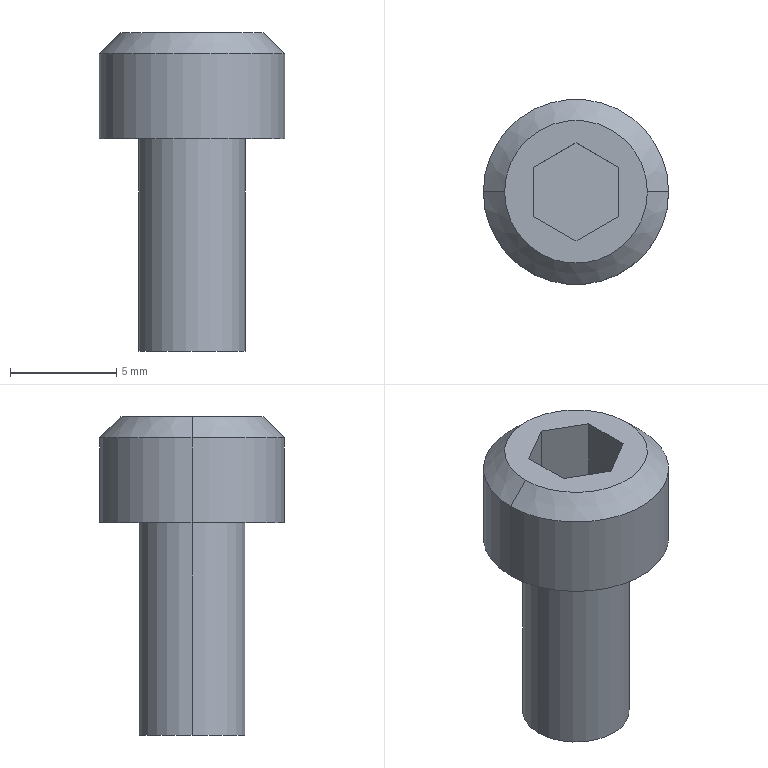Part | SolidWorks | features ICE 2, Chamfer 1, Extrusion 1 | 1 solid | 16 faces | box 8.72 x 8.72 x 15 mm | volume 426.876 mm3 | plane 10 | cylinder 4 | cone 2 | commonest cylinder face diameters 5 x2 8.72 x2
STEP:
#1=CARTESIAN_POINT('',(-2.5,0.,-10.));
#2=VERTEX_POINT('',#1);
#3=CARTESIAN_POINT('',(2.5,0.,-10.));
#4=VERTEX_POINT('',#3);
#5=CARTESIAN_POINT('',(0.,0.,-10.));
#6=DIRECTION('',(0.,0.,-1.));
#7=DIRECTION('',(-1.,0.,0.));
#8=AXIS2_PLACEMENT_3D('',#5,#6,#7);
#9=CIRCLE('',#8,2.5);
#10=EDGE_CURVE('',#2,#4,#9,.T.);
#11=ORIENTED_EDGE('',*,*,#10,.F.);
#12=CARTESIAN_POINT('',(-2.5,0.,0.));
#13=VERTEX_POINT('',#12);
#14=CARTESIAN_POINT('',(-2.5,0.,-10.));
#15=DIRECTION('',(0.,0.,1.));
#16=VECTOR('',#15,1000.);
#17=LINE('',#14,#16);
#18=EDGE_CURVE('',#2,#13,#17,.T.);
#19=ORIENTED_EDGE('',*,*,#18,.T.);
#20=CARTESIAN_POINT('',(2.5,0.,0.));
#21=VERTEX_POINT('',#20);
#22=CARTESIAN_POINT('',(0.,0.,0.));
#23=DIRECTION('',(0.,0.,-1.));
#24=DIRECTION('',(1.,0.,0.));
#25=AXIS2_PLACEMENT_3D('',#22,#23,#24);
#26=CIRCLE('',#25,2.5);
#27=EDGE_CURVE('',#13,#21,#26,.T.);
#28=ORIENTED_EDGE('',*,*,#27,.T.);
#29=CARTESIAN_POINT('',(2.5,0.,-10.));
#30=DIRECTION('',(0.,0.,1.));
#31=VECTOR('',#30,1000.);
#32=LINE('',#29,#31);
#33=EDGE_CURVE('',#4,#21,#32,.T.);
#34=ORIENTED_EDGE('',*,*,#33,.F.);
#35=EDGE_LOOP('',(#11,#19,#28,#34));
#36=FACE_OUTER_BOUND('',#35,.T.);
#37=CARTESIAN_POINT('',(0.,0.,-10.));
#38=DIRECTION('',(0.,0.,1.));
#39=DIRECTION('',(1.,0.,0.));
#40=AXIS2_PLACEMENT_3D('',#37,#38,#39);
#41=CYLINDRICAL_SURFACE('',#40,2.5);
#42=ADVANCED_FACE('',(#36),#41,.T.);
#43=CARTESIAN_POINT('',(3.36,0.,5.));
#44=VERTEX_POINT('',#43);
#45=CARTESIAN_POINT('',(-3.36,0.,5.));
#46=VERTEX_POINT('',#45);
#47=CARTESIAN_POINT('',(0.,0.,5.));
#48=DIRECTION('',(0.,0.,1.));
#49=DIRECTION('',(1.,0.,0.));
#50=AXIS2_PLACEMENT_3D('',#47,#48,#49);
#51=CIRCLE('',#50,3.36);
#52=EDGE_CURVE('',#44,#46,#51,.T.);
#53=ORIENTED_EDGE('',*,*,#52,.F.);
#54=CARTESIAN_POINT('',(4.36,0.,4.));
#55=VERTEX_POINT('',#54);
#56=CARTESIAN_POINT('',(3.36,0.,5.));
#57=DIRECTION('',(0.7071,0.,-0.7071));
#58=VECTOR('',#57,1000.);
#59=LINE('',#56,#58);
#60=EDGE_CURVE('',#44,#55,#59,.T.);
#61=ORIENTED_EDGE('',*,*,#60,.T.);
#62=CARTESIAN_POINT('',(-4.36,0.,4.));
#63=VERTEX_POINT('',#62);
#64=CARTESIAN_POINT('',(0.,0.,4.));
#65=DIRECTION('',(0.,0.,-1.));
#66=DIRECTION('',(1.,0.,0.));
#67=AXIS2_PLACEMENT_3D('',#64,#65,#66);
#68=CIRCLE('',#67,4.36);
#69=EDGE_CURVE('',#63,#55,#68,.T.);
#70=ORIENTED_EDGE('',*,*,#69,.F.);
#71=CARTESIAN_POINT('',(-3.36,0.,5.));
#72=DIRECTION('',(-0.7071,0.,-0.7071));
#73=VECTOR('',#72,1000.);
#74=LINE('',#71,#73);
#75=EDGE_CURVE('',#46,#63,#74,.T.);
#76=ORIENTED_EDGE('',*,*,#75,.F.);
#77=EDGE_LOOP('',(#53,#61,#70,#76));
#78=FACE_OUTER_BOUND('',#77,.T.);
#79=CARTESIAN_POINT('',(0.,0.,5.));
#80=DIRECTION('',(0.,0.,-1.));
#81=DIRECTION('',(-1.,0.,0.));
#82=AXIS2_PLACEMENT_3D('',#79,#80,#81);
#83=CONICAL_SURFACE('',#82,3.36,0.7854);
#84=ADVANCED_FACE('',(#78),#83,.T.);
#85=ORIENTED_EDGE('',*,*,#69,.T.);
#86=CARTESIAN_POINT('',(4.36,0.,0.));
#87=VERTEX_POINT('',#86);
#88=CARTESIAN_POINT('',(4.36,0.,5.));
#89=DIRECTION('',(0.,0.,-1.));
#90=VECTOR('',#89,1000.);
#91=LINE('',#88,#90);
#92=EDGE_CURVE('',#55,#87,#91,.T.);
#93=ORIENTED_EDGE('',*,*,#92,.T.);
#94=CARTESIAN_POINT('',(-4.36,0.,0.));
#95=VERTEX_POINT('',#94);
#96=CARTESIAN_POINT('',(0.,0.,0.));
#97=DIRECTION('',(0.,0.,1.));
#98=DIRECTION('',(1.,0.,0.));
#99=AXIS2_PLACEMENT_3D('',#96,#97,#98);
#100=CIRCLE('',#99,4.36);
#101=EDGE_CURVE('',#87,#95,#100,.T.);
#102=ORIENTED_EDGE('',*,*,#101,.T.);
#103=CARTESIAN_POINT('',(-4.36,0.,5.));
#104=DIRECTION('',(0.,0.,-1.));
#105=VECTOR('',#104,1000.);
#106=LINE('',#103,#105);
#107=EDGE_CURVE('',#63,#95,#106,.T.);
#108=ORIENTED_EDGE('',*,*,#107,.F.);
#109=EDGE_LOOP('',(#85,#93,#102,#108));
#110=FACE_OUTER_BOUND('',#109,.T.);
#111=CARTESIAN_POINT('',(0.,0.,5.));
#112=DIRECTION('',(0.,0.,-1.));
#113=DIRECTION('',(-1.,0.,0.));
#114=AXIS2_PLACEMENT_3D('',#111,#112,#113);
#115=CYLINDRICAL_SURFACE('',#114,4.36);
#116=ADVANCED_FACE('',(#110),#115,.T.);
#117=CARTESIAN_POINT('',(0.,0.,0.));
#118=DIRECTION('',(0.,0.,1.));
#119=DIRECTION('',(1.,0.,0.));
#120=AXIS2_PLACEMENT_3D('',#117,#118,#119);
#121=CIRCLE('',#120,4.36);
#122=EDGE_CURVE('',#95,#87,#121,.T.);
#123=ORIENTED_EDGE('',*,*,#122,.F.);
#124=ORIENTED_EDGE('',*,*,#101,.F.);
#125=EDGE_LOOP('',(#123,#124));
#126=FACE_OUTER_BOUND('',#125,.T.);
#127=CARTESIAN_POINT('',(0.,0.,0.));
#128=DIRECTION('',(0.,0.,-1.));
#129=DIRECTION('',(1.,0.,0.));
#130=AXIS2_PLACEMENT_3D('',#127,#128,#129);
#131=CIRCLE('',#130,2.5);
#132=EDGE_CURVE('',#21,#13,#131,.T.);
#133=ORIENTED_EDGE('',*,*,#132,.F.);
#134=ORIENTED_EDGE('',*,*,#27,.F.);
#135=EDGE_LOOP('',(#133,#134));
#136=FACE_BOUND('',#135,.T.);
#137=CARTESIAN_POINT('',(0.,0.,0.));
#138=DIRECTION('',(0.,0.,1.));
#139=DIRECTION('',(1.,0.,0.));
#140=AXIS2_PLACEMENT_3D('',#137,#138,#139);
#141=PLANE('',#140);
#142=ADVANCED_FACE('',(#126,#136),#141,.F.);
#143=ORIENTED_EDGE('',*,*,#92,.F.);
#144=CARTESIAN_POINT('',(0.,0.,4.));
#145=DIRECTION('',(0.,0.,-1.));
#146=DIRECTION('',(1.,0.,0.));
#147=AXIS2_PLACEMENT_3D('',#144,#145,#146);
#148=CIRCLE('',#147,4.36);
#149=EDGE_CURVE('',#55,#63,#148,.T.);
#150=ORIENTED_EDGE('',*,*,#149,.T.);
#151=ORIENTED_EDGE('',*,*,#107,.T.);
#152=ORIENTED_EDGE('',*,*,#122,.T.);
#153=EDGE_LOOP('',(#143,#150,#151,#152));
#154=FACE_OUTER_BOUND('',#153,.T.);
#155=CARTESIAN_POINT('',(0.,0.,5.));
#156=DIRECTION('',(0.,0.,-1.));
#157=DIRECTION('',(-1.,0.,0.));
#158=AXIS2_PLACEMENT_3D('',#155,#156,#157);
#159=CYLINDRICAL_SURFACE('',#158,4.36);
#160=ADVANCED_FACE('',(#154),#159,.T.);
#161=CARTESIAN_POINT('',(0.,0.,5.));
#162=DIRECTION('',(0.,0.,1.));
#163=DIRECTION('',(1.,0.,0.));
#164=AXIS2_PLACEMENT_3D('',#161,#162,#163);
#165=CIRCLE('',#164,3.36);
#166=EDGE_CURVE('',#46,#44,#165,.T.);
#167=ORIENTED_EDGE('',*,*,#166,.T.);
#168=ORIENTED_EDGE('',*,*,#52,.T.);
#169=EDGE_LOOP('',(#167,#168));
#170=FACE_OUTER_BOUND('',#169,.T.);
#171=CARTESIAN_POINT('',(2.,1.155,5.));
#172=VERTEX_POINT('',#171);
#173=CARTESIAN_POINT('',(0.,2.309,5.));
#174=VERTEX_POINT('',#173);
#175=CARTESIAN_POINT('',(2.,1.155,5.));
#176=DIRECTION('',(-0.866,0.5,0.));
#177=VECTOR('',#176,1000.);
#178=LINE('',#175,#177);
#179=EDGE_CURVE('',#172,#174,#178,.T.);
#180=ORIENTED_EDGE('',*,*,#179,.F.);
#181=CARTESIAN_POINT('',(2.,-1.155,5.));
#182=VERTEX_POINT('',#181);
#183=CARTESIAN_POINT('',(2.,-1.155,5.));
#184=DIRECTION('',(0.,1.,0.));
#185=VECTOR('',#184,1000.);
#186=LINE('',#183,#185);
#187=EDGE_CURVE('',#182,#172,#186,.T.);
#188=ORIENTED_EDGE('',*,*,#187,.F.);
#189=CARTESIAN_POINT('',(0.,-2.309,5.));
#190=VERTEX_POINT('',#189);
#191=CARTESIAN_POINT('',(0.,-2.309,5.));
#192=DIRECTION('',(0.866,0.5,0.));
#193=VECTOR('',#192,1000.);
#194=LINE('',#191,#193);
#195=EDGE_CURVE('',#190,#182,#194,.T.);
#196=ORIENTED_EDGE('',*,*,#195,.F.);
#197=CARTESIAN_POINT('',(-2.,-1.155,5.));
#198=VERTEX_POINT('',#197);
#199=CARTESIAN_POINT('',(-2.,-1.155,5.));
#200=DIRECTION('',(0.866,-0.5,0.));
#201=VECTOR('',#200,1000.);
#202=LINE('',#199,#201);
#203=EDGE_CURVE('',#198,#190,#202,.T.);
#204=ORIENTED_EDGE('',*,*,#203,.F.);
#205=CARTESIAN_POINT('',(-2.,1.155,5.));
#206=VERTEX_POINT('',#205);
#207=CARTESIAN_POINT('',(-2.,1.155,5.));
#208=DIRECTION('',(0.,-1.,0.));
#209=VECTOR('',#208,1000.);
#210=LINE('',#207,#209);
#211=EDGE_CURVE('',#206,#198,#210,.T.);
#212=ORIENTED_EDGE('',*,*,#211,.F.);
#213=CARTESIAN_POINT('',(0.,2.309,5.));
#214=DIRECTION('',(-0.866,-0.5,0.));
#215=VECTOR('',#214,1000.);
#216=LINE('',#213,#215);
#217=EDGE_CURVE('',#174,#206,#216,.T.);
#218=ORIENTED_EDGE('',*,*,#217,.F.);
#219=EDGE_LOOP('',(#180,#188,#196,#204,#212,#218));
#220=FACE_BOUND('',#219,.T.);
#221=CARTESIAN_POINT('',(0.,0.,5.));
#222=DIRECTION('',(0.,0.,1.));
#223=DIRECTION('',(1.,0.,0.));
#224=AXIS2_PLACEMENT_3D('',#221,#222,#223);
#225=PLANE('',#224);
#226=ADVANCED_FACE('',(#170,#220),#225,.T.);
#227=ORIENTED_EDGE('',*,*,#179,.T.);
#228=CARTESIAN_POINT('',(0.,2.309,1.));
#229=VERTEX_POINT('',#228);
#230=CARTESIAN_POINT('',(0.,2.309,1.));
#231=DIRECTION('',(0.,0.,1.));
#232=VECTOR('',#231,1000.);
#233=LINE('',#230,#232);
#234=EDGE_CURVE('',#229,#174,#233,.T.);
#235=ORIENTED_EDGE('',*,*,#234,.F.);
#236=CARTESIAN_POINT('',(2.,1.155,1.));
#237=VERTEX_POINT('',#236);
#238=CARTESIAN_POINT('',(2.,1.155,1.));
#239=DIRECTION('',(-0.866,0.5,0.));
#240=VECTOR('',#239,1000.);
#241=LINE('',#238,#240);
#242=EDGE_CURVE('',#237,#229,#241,.T.);
#243=ORIENTED_EDGE('',*,*,#242,.F.);
#244=CARTESIAN_POINT('',(2.,1.155,1.));
#245=DIRECTION('',(0.,0.,1.));
#246=VECTOR('',#245,1000.);
#247=LINE('',#244,#246);
#248=EDGE_CURVE('',#237,#172,#247,.T.);
#249=ORIENTED_EDGE('',*,*,#248,.T.);
#250=EDGE_LOOP('',(#227,#235,#243,#249));
#251=FACE_OUTER_BOUND('',#250,.T.);
#252=CARTESIAN_POINT('',(2.,1.155,1.));
#253=DIRECTION('',(0.5,0.866,0.));
#254=DIRECTION('',(-0.866,0.5,0.));
#255=AXIS2_PLACEMENT_3D('',#252,#253,#254);
#256=PLANE('',#255);
#257=ADVANCED_FACE('',(#251),#256,.F.);
#258=ORIENTED_EDGE('',*,*,#187,.T.);
#259=ORIENTED_EDGE('',*,*,#248,.F.);
#260=CARTESIAN_POINT('',(2.,-1.155,1.));
#261=VERTEX_POINT('',#260);
#262=CARTESIAN_POINT('',(2.,-1.155,1.));
#263=DIRECTION('',(0.,1.,0.));
#264=VECTOR('',#263,1000.);
#265=LINE('',#262,#264);
#266=EDGE_CURVE('',#261,#237,#265,.T.);
#267=ORIENTED_EDGE('',*,*,#266,.F.);
#268=CARTESIAN_POINT('',(2.,-1.155,1.));
#269=DIRECTION('',(0.,0.,1.));
#270=VECTOR('',#269,1000.);
#271=LINE('',#268,#270);
#272=EDGE_CURVE('',#261,#182,#271,.T.);
#273=ORIENTED_EDGE('',*,*,#272,.T.);
#274=EDGE_LOOP('',(#258,#259,#267,#273));
#275=FACE_OUTER_BOUND('',#274,.T.);
#276=CARTESIAN_POINT('',(2.,-1.155,1.));
#277=DIRECTION('',(1.,0.,0.));
#278=DIRECTION('',(0.,1.,0.));
#279=AXIS2_PLACEMENT_3D('',#276,#277,#278);
#280=PLANE('',#279);
#281=ADVANCED_FACE('',(#275),#280,.F.);
#282=ORIENTED_EDGE('',*,*,#195,.T.);
#283=ORIENTED_EDGE('',*,*,#272,.F.);
#284=CARTESIAN_POINT('',(0.,-2.309,1.));
#285=VERTEX_POINT('',#284);
#286=CARTESIAN_POINT('',(0.,-2.309,1.));
#287=DIRECTION('',(0.866,0.5,0.));
#288=VECTOR('',#287,1000.);
#289=LINE('',#286,#288);
#290=EDGE_CURVE('',#285,#261,#289,.T.);
#291=ORIENTED_EDGE('',*,*,#290,.F.);
#292=CARTESIAN_POINT('',(0.,-2.309,1.));
#293=DIRECTION('',(0.,0.,1.));
#294=VECTOR('',#293,1000.);
#295=LINE('',#292,#294);
#296=EDGE_CURVE('',#285,#190,#295,.T.);
#297=ORIENTED_EDGE('',*,*,#296,.T.);
#298=EDGE_LOOP('',(#282,#283,#291,#297));
#299=FACE_OUTER_BOUND('',#298,.T.);
#300=CARTESIAN_POINT('',(0.,-2.309,1.));
#301=DIRECTION('',(0.5,-0.866,0.));
#302=DIRECTION('',(0.866,0.5,0.));
#303=AXIS2_PLACEMENT_3D('',#300,#301,#302);
#304=PLANE('',#303);
#305=ADVANCED_FACE('',(#299),#304,.F.);
#306=ORIENTED_EDGE('',*,*,#203,.T.);
#307=ORIENTED_EDGE('',*,*,#296,.F.);
#308=CARTESIAN_POINT('',(-2.,-1.155,1.));
#309=VERTEX_POINT('',#308);
#310=CARTESIAN_POINT('',(-2.,-1.155,1.));
#311=DIRECTION('',(0.866,-0.5,0.));
#312=VECTOR('',#311,1000.);
#313=LINE('',#310,#312);
#314=EDGE_CURVE('',#309,#285,#313,.T.);
#315=ORIENTED_EDGE('',*,*,#314,.F.);
#316=CARTESIAN_POINT('',(-2.,-1.155,1.));
#317=DIRECTION('',(0.,0.,1.));
#318=VECTOR('',#317,1000.);
#319=LINE('',#316,#318);
#320=EDGE_CURVE('',#309,#198,#319,.T.);
#321=ORIENTED_EDGE('',*,*,#320,.T.);
#322=EDGE_LOOP('',(#306,#307,#315,#321));
#323=FACE_OUTER_BOUND('',#322,.T.);
#324=CARTESIAN_POINT('',(-2.,-1.155,1.));
#325=DIRECTION('',(-0.5,-0.866,0.));
#326=DIRECTION('',(0.866,-0.5,0.));
#327=AXIS2_PLACEMENT_3D('',#324,#325,#326);
#328=PLANE('',#327);
#329=ADVANCED_FACE('',(#323),#328,.F.);
#330=ORIENTED_EDGE('',*,*,#211,.T.);
#331=ORIENTED_EDGE('',*,*,#320,.F.);
#332=CARTESIAN_POINT('',(-2.,1.155,1.));
#333=VERTEX_POINT('',#332);
#334=CARTESIAN_POINT('',(-2.,1.155,1.));
#335=DIRECTION('',(0.,-1.,0.));
#336=VECTOR('',#335,1000.);
#337=LINE('',#334,#336);
#338=EDGE_CURVE('',#333,#309,#337,.T.);
#339=ORIENTED_EDGE('',*,*,#338,.F.);
#340=CARTESIAN_POINT('',(-2.,1.155,1.));
#341=DIRECTION('',(0.,0.,1.));
#342=VECTOR('',#341,1000.);
#343=LINE('',#340,#342);
#344=EDGE_CURVE('',#333,#206,#343,.T.);
#345=ORIENTED_EDGE('',*,*,#344,.T.);
#346=EDGE_LOOP('',(#330,#331,#339,#345));
#347=FACE_OUTER_BOUND('',#346,.T.);
#348=CARTESIAN_POINT('',(-2.,1.155,1.));
#349=DIRECTION('',(-1.,0.,0.));
#350=DIRECTION('',(0.,0.,1.));
#351=AXIS2_PLACEMENT_3D('',#348,#349,#350);
#352=PLANE('',#351);
#353=ADVANCED_FACE('',(#347),#352,.F.);
#354=ORIENTED_EDGE('',*,*,#217,.T.);
#355=ORIENTED_EDGE('',*,*,#344,.F.);
#356=CARTESIAN_POINT('',(0.,2.309,1.));
#357=DIRECTION('',(-0.866,-0.5,0.));
#358=VECTOR('',#357,1000.);
#359=LINE('',#356,#358);
#360=EDGE_CURVE('',#229,#333,#359,.T.);
#361=ORIENTED_EDGE('',*,*,#360,.F.);
#362=ORIENTED_EDGE('',*,*,#234,.T.);
#363=EDGE_LOOP('',(#354,#355,#361,#362));
#364=FACE_OUTER_BOUND('',#363,.T.);
#365=CARTESIAN_POINT('',(0.,2.309,1.));
#366=DIRECTION('',(-0.5,0.866,0.));
#367=DIRECTION('',(-0.866,-0.5,0.));
#368=AXIS2_PLACEMENT_3D('',#365,#366,#367);
#369=PLANE('',#368);
#370=ADVANCED_FACE('',(#364),#369,.F.);
#371=ORIENTED_EDGE('',*,*,#242,.T.);
#372=ORIENTED_EDGE('',*,*,#360,.T.);
#373=ORIENTED_EDGE('',*,*,#338,.T.);
#374=ORIENTED_EDGE('',*,*,#314,.T.);
#375=ORIENTED_EDGE('',*,*,#290,.T.);
#376=ORIENTED_EDGE('',*,*,#266,.T.);
#377=EDGE_LOOP('',(#371,#372,#373,#374,#375,#376));
#378=FACE_OUTER_BOUND('',#377,.T.);
#379=CARTESIAN_POINT('',(0.,0.,1.));
#380=DIRECTION('',(0.,0.,1.));
#381=DIRECTION('',(1.,0.,0.));
#382=AXIS2_PLACEMENT_3D('',#379,#380,#381);
#383=PLANE('',#382);
#384=ADVANCED_FACE('',(#378),#383,.T.);
#385=ORIENTED_EDGE('',*,*,#60,.F.);
#386=ORIENTED_EDGE('',*,*,#166,.F.);
#387=ORIENTED_EDGE('',*,*,#75,.T.);
#388=ORIENTED_EDGE('',*,*,#149,.F.);
#389=EDGE_LOOP('',(#385,#386,#387,#388));
#390=FACE_OUTER_BOUND('',#389,.T.);
#391=CARTESIAN_POINT('',(0.,0.,5.));
#392=DIRECTION('',(0.,0.,-1.));
#393=DIRECTION('',(-1.,0.,0.));
#394=AXIS2_PLACEMENT_3D('',#391,#392,#393);
#395=CONICAL_SURFACE('',#394,3.36,0.7854);
#396=ADVANCED_FACE('',(#390),#395,.T.);
#397=ORIENTED_EDGE('',*,*,#18,.F.);
#398=CARTESIAN_POINT('',(0.,0.,-10.));
#399=DIRECTION('',(0.,0.,-1.));
#400=DIRECTION('',(-1.,0.,0.));
#401=AXIS2_PLACEMENT_3D('',#398,#399,#400);
#402=CIRCLE('',#401,2.5);
#403=EDGE_CURVE('',#4,#2,#402,.T.);
#404=ORIENTED_EDGE('',*,*,#403,.F.);
#405=ORIENTED_EDGE('',*,*,#33,.T.);
#406=ORIENTED_EDGE('',*,*,#132,.T.);
#407=EDGE_LOOP('',(#397,#404,#405,#406));
#408=FACE_OUTER_BOUND('',#407,.T.);
#409=CARTESIAN_POINT('',(0.,0.,-10.));
#410=DIRECTION('',(0.,0.,1.));
#411=DIRECTION('',(1.,0.,0.));
#412=AXIS2_PLACEMENT_3D('',#409,#410,#411);
#413=CYLINDRICAL_SURFACE('',#412,2.5);
#414=ADVANCED_FACE('',(#408),#413,.T.);
#415=ORIENTED_EDGE('',*,*,#403,.T.);
#416=ORIENTED_EDGE('',*,*,#10,.T.);
#417=EDGE_LOOP('',(#415,#416));
#418=FACE_OUTER_BOUND('',#417,.T.);
#419=CARTESIAN_POINT('',(0.,0.,-10.));
#420=DIRECTION('',(0.,0.,-1.));
#421=DIRECTION('',(-1.,0.,0.));
#422=AXIS2_PLACEMENT_3D('',#419,#420,#421);
#423=PLANE('',#422);
#424=ADVANCED_FACE('',(#418),#423,.T.);
#425=CLOSED_SHELL('',(#42,#84,#116,#142,#160,#226,#257,#281,#305,#329,#353,#370,#384,#396,#414,#424));
#426=MANIFOLD_SOLID_BREP('',#425);
#427=CARTESIAN_POINT('',(0.,0.,0.));
#428=DIRECTION('',(0.,0.,1.));
#429=DIRECTION('',(1.,0.,0.));
#430=AXIS2_PLACEMENT_3D('',#427,#428,#429);
#431=(LENGTH_UNIT()NAMED_UNIT(*)SI_UNIT(.MILLI.,.METRE.));
#432=UNCERTAINTY_MEASURE_WITH_UNIT(LENGTH_MEASURE(0.00001),#431,'','');
#433=(NAMED_UNIT(*)PLANE_ANGLE_UNIT()SI_UNIT($,.RADIAN.));
#434=(NAMED_UNIT(*)SI_UNIT($,.STERADIAN.)SOLID_ANGLE_UNIT());
#435=(GEOMETRIC_REPRESENTATION_CONTEXT(3)GLOBAL_UNCERTAINTY_ASSIGNED_CONTEXT((#432))GLOBAL_UNIT_ASSIGNED_CONTEXT((#431,#433,#434))REPRESENTATION_CONTEXT('',''));
#436=ADVANCED_BREP_SHAPE_REPRESENTATION('',(#426,#430),#435);